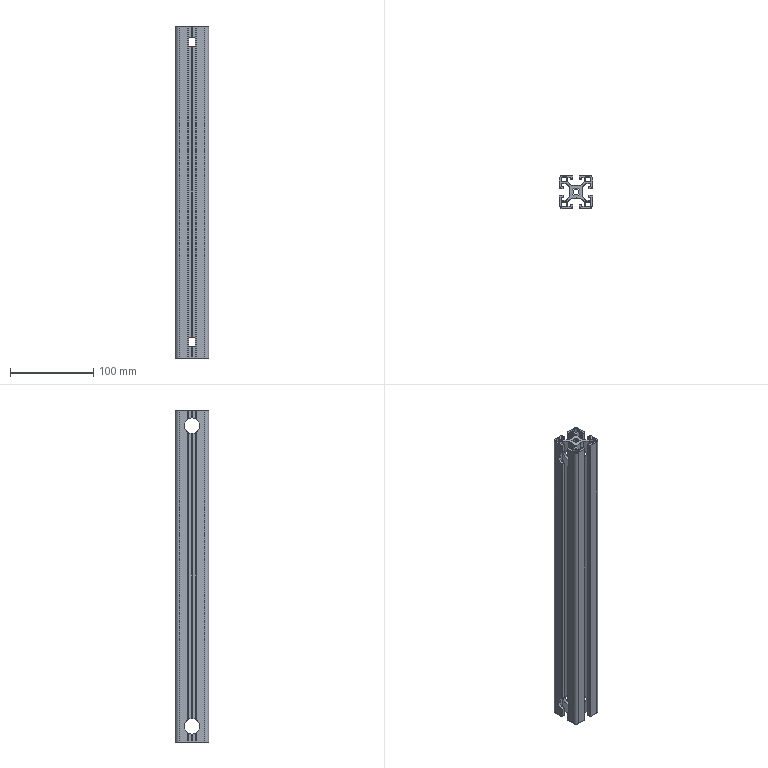Part | SolidWorks | features Extrusion 1, HoleWzd 1 | 1 solid | 273 faces | box 40 x 40 x 400 mm | volume 232057 mm3 | plane 213 | cylinder 60 | commonest cylinder face diameters 2 x16 6.8 x15 19 x12 1 x8 5 x4 9 x4